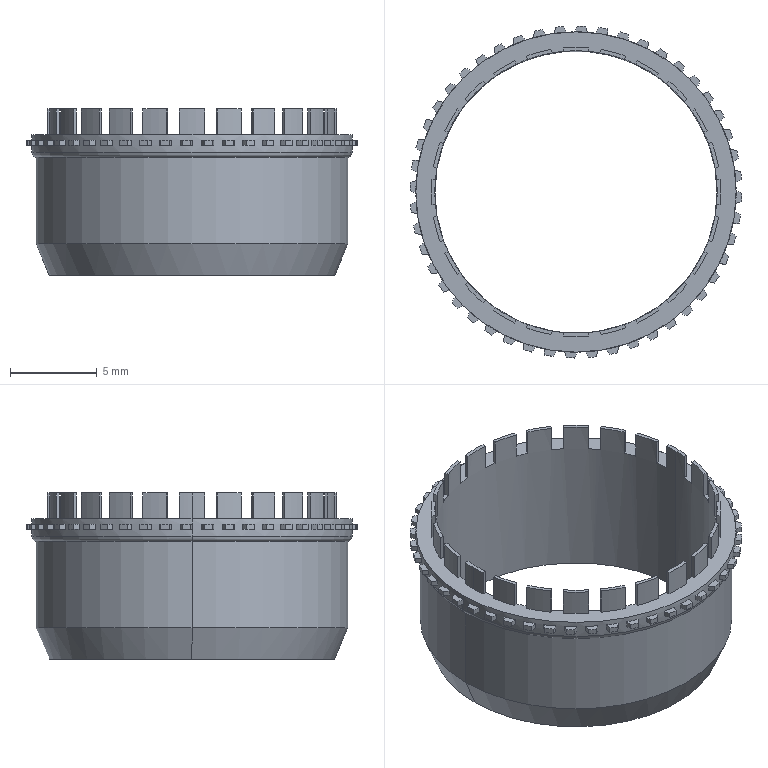Part | SolidWorks | features ICE 5, CirPattern 2, Blend 1, Extrusion 1, Fillet 1 | 1 solid | 351 faces | box 19.179 x 19.179 x 9.6 mm | volume 364.987 mm3 | cylinder 177 | plane 170 | torus 2 | cone 2 | commonest cylinder face diameters 6.431 x98 19.18 x48 16.71 x25 16.3 x2 18 x2 18.5 x2